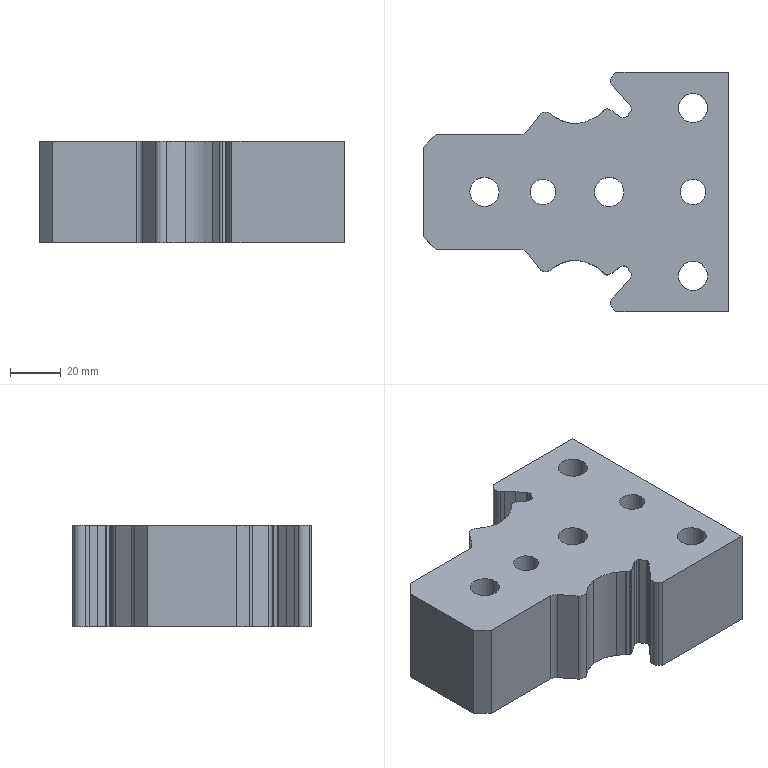Part | NX | features 8 2 | 1 solid | 78 faces | box 120 x 94 x 40 mm | volume 281283 mm3 | plane 36 | cylinder 24 | spline 18 | commonest cylinder face diameters 6 x6 4 x4 11.5 x4 18 x4 10.001 x2 10.31 x2